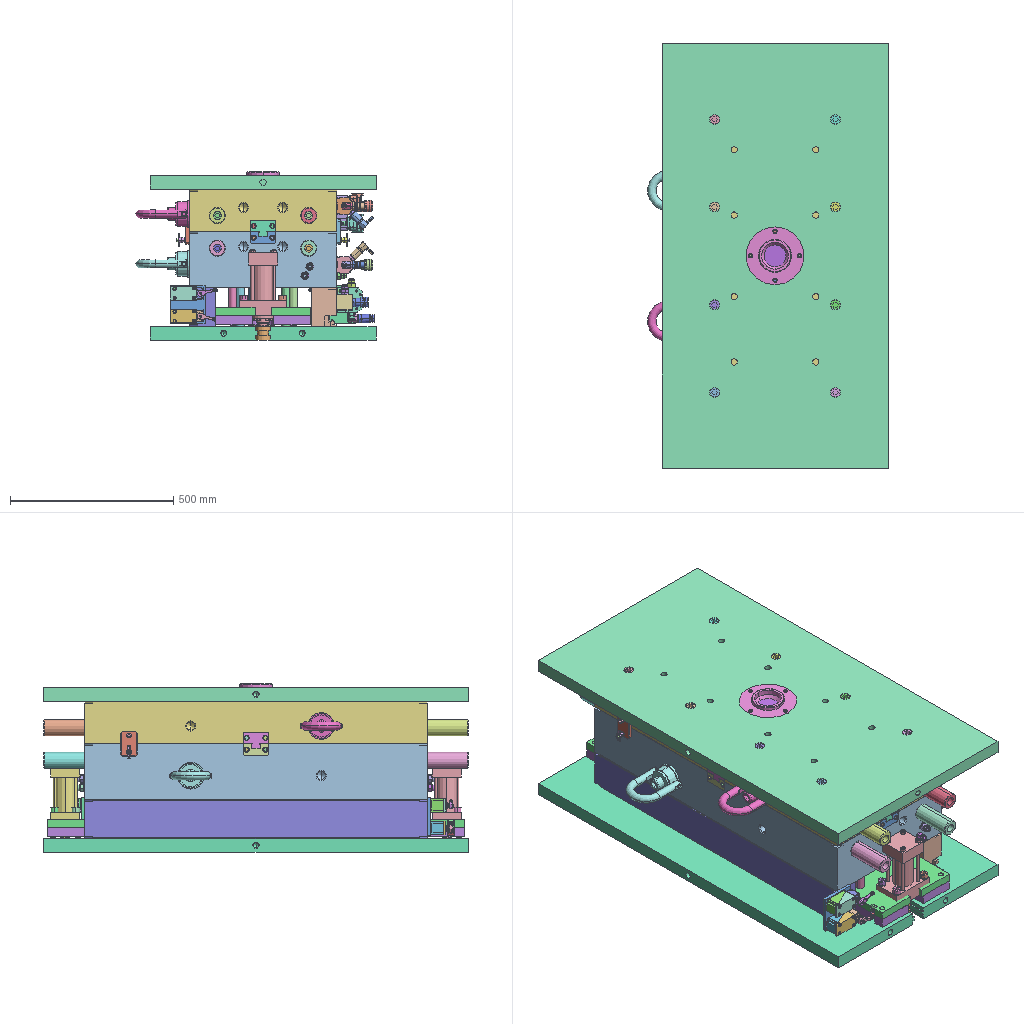Assembly | STEP file | 442 different items | 442 placed | box 735 x 1300 x 515 mm
Parts list (item | name | quantity | parent item | size | volume), first 288 of 442 items:
1 | 1 | x1 | in 4-20 | 615.081 x 1049 x 462.275 mm | 3467998 mm3
2 | 4-20.sldasm-Part-1 (subassembly) | x1 | in 4-20 | 46.6 x 158.128 x 57 mm | 97175 mm3
3 | 4-20.sldasm-Part-10 (subassembly) | x1 | in 4-20 | 14 x 7 x 7 mm | 262.874 mm3
4 | 4-20.sldasm-Part-100 (subassembly) | x1 | in 4-20 | 45.212 x 25.216 x 24.222 mm | 9310 mm3
5 | 4-20.sldasm-Part-101 (subassembly) | x1 | in 4-20 | 50 x 80 x 50 mm | 195848 mm3
6 | 4-20.sldasm-Part-102 (subassembly) | x1 | in 4-20 | 23.812 x 23.812 x 85.725 mm | 19411 mm3
7 | 4-20.sldasm-Part-103 (subassembly) | x1 | in 4-20 | 23.813 x 23.812 x 85.725 mm | 19411 mm3
8 | 4-20.sldasm-Part-104 (subassembly) | x1 | in 4-20 | 110 x 9.525 x 9.525 mm | 7838 mm3
9 | 4-20.sldasm-Part-105 (subassembly) | x1 | in 4-20 | 9.525 x 1050 x 9.525 mm | 74819 mm3
10 | 4-20.sldasm-Part-106 (subassembly) | x1 | in 4-20 | 23 x 10 x 10 mm | 863.941 mm3
11 | 4-20.sldasm-Part-107 (subassembly) | x1 | in 4-20 | 23.813 x 23.812 x 85.725 mm | 19411 mm3
12 | 4-20.sldasm-Part-108 (subassembly) | x1 | in 4-20 | 95 x 9.525 x 9.525 mm | 6769 mm3
13 | 4-20.sldasm-Part-109 (subassembly) | x1 | in 4-20 | 44.22 x 44.22 x 41.275 mm | 38759 mm3
14 | 4-20.sldasm-Part-11 (subassembly) | x1 | in 4-20 | 46.6 x 118.128 x 57 mm | 74877 mm3
15 | 4-20.sldasm-Part-110 (subassembly) | x1 | in 4-20 | 25.216 x 45.212 x 24.222 mm | 9310 mm3
16 | 4-20.sldasm-Part-111 (subassembly) | x1 | in 4-20 | 45.212 x 25.216 x 24.222 mm | 9310 mm3
17 | 4-20.sldasm-Part-112 (subassembly) | x1 | in 4-20 | 95 x 9.525 x 9.525 mm | 6769 mm3
18 | 4-20.sldasm-Part-113 (subassembly) | x1 | in 4-20 | 23 x 10 x 10 mm | 863.941 mm3
19 | 4-20.sldasm-Part-114 (subassembly) | x1 | in 4-20 | 23.813 x 23.812 x 85.725 mm | 19411 mm3
20 | 4-20.sldasm-Part-115 (subassembly) | x1 | in 4-20 | 25.216 x 45.212 x 24.222 mm | 9310 mm3
21 | 4-20.sldasm-Part-116 (subassembly) | x1 | in 4-20 | 25.216 x 45.212 x 24.222 mm | 9310 mm3
22 | 4-20.sldasm-Part-117 (subassembly) | x1 | in 4-20 | 23.813 x 23.812 x 85.725 mm | 19411 mm3
23 | 4-20.sldasm-Part-118 (subassembly) | x1 | in 4-20 | 50 x 29.094 x 26 mm | 17659 mm3
24 | 4-20.sldasm-Part-119 (subassembly) | x1 | in 4-20 | 24.222 x 25.216 x 45.212 mm | 9310 mm3
25 | 4-20.sldasm-Part-12 (subassembly) | x1 | in 4-20 | 14 x 7 x 7 mm | 262.874 mm3
26 | 4-20.sldasm-Part-120 (subassembly) | x1 | in 4-20 | 23.813 x 23.812 x 85.725 mm | 19411 mm3
27 | 4-20.sldasm-Part-121 (subassembly) | x1 | in 4-20 | 45.212 x 25.216 x 24.222 mm | 9310 mm3
28 | 4-20.sldasm-Part-122 (subassembly) | x1 | in 4-20 | 22.225 x 25.663 x 45.212 mm | 9310 mm3
29 | 4-20.sldasm-Part-123 (subassembly) | x1 | in 4-20 | 24.222 x 25.216 x 45.212 mm | 9310 mm3
30 | 4-20.sldasm-Part-124 (subassembly) | x1 | in 4-20 | 23.813 x 23.812 x 85.725 mm | 19411 mm3
31 | 4-20.sldasm-Part-125 (subassembly) | x1 | in 4-20 | 142.875 x 88.9 x 276.19 mm | 1282545 mm3
32 | 4-20.sldasm-Part-126 (subassembly) | x1 | in 4-20 | 44.22 x 44.22 x 41.275 mm | 38759 mm3
33 | 4-20.sldasm-Part-127 (subassembly) | x1 | in 4-20 | 22.225 x 25.663 x 45.212 mm | 9310 mm3
34 | 4-20.sldasm-Part-128 (subassembly) | x1 | in 4-20 | 45 x 22 x 45 mm | 14976 mm3
35 | 4-20.sldasm-Part-129 (subassembly) | x1 | in 4-20 | 79 x 192 x 94.5 mm | 576073 mm3
36 | 4-20.sldasm-Part-13 (subassembly) | x1 | in 4-20 | 14 x 7 x 7 mm | 262.874 mm3
37 | 4-20.sldasm-Part-130 (subassembly) | x1 | in 4-20 | 23 x 10 x 10 mm | 863.941 mm3
38 | 4-20.sldasm-Part-131 (subassembly) | x1 | in 4-20 | 25.216 x 45.212 x 24.222 mm | 9310 mm3
39 | 4-20.sldasm-Part-132 (subassembly) | x1 | in 4-20 | 23 x 10 x 10 mm | 863.941 mm3
40 | 4-20.sldasm-Part-133 (subassembly) | x1 | in 4-20 | 45 x 45 x 22 mm | 14976 mm3
41 | 4-20.sldasm-Part-134 (subassembly) | x1 | in 4-20 | 45.212 x 25.216 x 24.222 mm | 9310 mm3
42 | 4-20.sldasm-Part-135 (subassembly) | x1 | in 4-20 | 142.875 x 88.9 x 276.19 mm | 1282545 mm3
43 | 4-20.sldasm-Part-136 (subassembly) | x1 | in 4-20 | 59 x 10 x 10 mm | 1882 mm3
44 | 4-20.sldasm-Part-137 (subassembly) | x1 | in 4-20 | 23.812 x 23.812 x 85.725 mm | 19411 mm3
45 | 4-20.sldasm-Part-138 (subassembly) | x1 | in 4-20 | 9.525 x 1050 x 9.525 mm | 74819 mm3
46 | 4-20.sldasm-Part-139 (subassembly) | x1 | in 4-20 | 50 x 32 x 32 mm | 24309 mm3
47 | 4-20.sldasm-Part-14 (subassembly) | x1 | in 4-20 | 20 x 100 x 43 mm | 85571 mm3
48 | 4-20.sldasm-Part-140 (subassembly) | x1 | in 4-20 | 110 x 9.525 x 9.525 mm | 7838 mm3
49 | 4-20.sldasm-Part-141 (subassembly) | x1 | in 4-20 | 8.306 x 5.45 x 5.45 mm | 72.235 mm3
50 | 4-20.sldasm-Part-142 (subassembly) | x1 | in 4-20 | 3.175 x 9.6 x 3.175 mm | 75.624 mm3
51 | 4-20.sldasm-Part-143 (subassembly) | x1 | in 4-20 | 12.1 x 3.3 x 12.1 mm | 339.506 mm3
52 | 4-20.sldasm-Part-144 (subassembly) | x1 | in 4-20 | 8.306 x 5.45 x 5.45 mm | 72.196 mm3
53 | 4-20.sldasm-Part-145 (subassembly) | x1 | in 4-20 | 11.112 x 56.8 x 11.112 mm | 2501 mm3
54 | 4-20.sldasm-Part-146 (subassembly) | x1 | in 4-20 | 3.175 x 9.6 x 3.175 mm | 75.624 mm3
55 | 4-20.sldasm-Part-147 (subassembly) | x1 | in 4-20 | 9.525 x 54.15 x 9.525 mm | 1881 mm3
56 | 4-20.sldasm-Part-148 (subassembly) | x1 | in 4-20 | 7.82 x 42.968 x 7.82 mm | 439.236 mm3
57 | 4-20.sldasm-Part-149 (subassembly) | x1 | in 4-20 | 22.225 x 45.05 x 34.95 mm | 29644 mm3
58 | 4-20.sldasm-Part-15 (subassembly) | x1 | in 4-20 | 71.345 x 25 x 55.031 mm | 25800 mm3
59 | 4-20.sldasm-Part-150 (subassembly) | x1 | in 4-20 | 8.306 x 5.45 x 5.45 mm | 72.235 mm3
60 | 4-20.sldasm-Part-151 (subassembly) | x1 | in 4-20 | 20 x 15.87 x 15.87 mm | 3956 mm3
61 | 4-20.sldasm-Part-152 (subassembly) | x1 | in 4-20 | 11.112 x 56.8 x 11.112 mm | 2501 mm3
62 | 4-20.sldasm-Part-153 (subassembly) | x1 | in 4-20 | 8.306 x 5.45 x 5.45 mm | 72.196 mm3
63 | 4-20.sldasm-Part-154 (subassembly) | x1 | in 4-20 | 6.35 x 17.375 x 6.35 mm | 540.618 mm3
64 | 4-20.sldasm-Part-155 (subassembly) | x1 | in 4-20 | 6.35 x 17.375 x 6.35 mm | 540.618 mm3
65 | 4-20.sldasm-Part-156 (subassembly) | x1 | in 4-20 | 8.306 x 5.45 x 5.45 mm | 72.196 mm3
66 | 4-20.sldasm-Part-157 (subassembly) | x1 | in 4-20 | 11.112 x 56.8 x 11.112 mm | 2501 mm3
67 | 4-20.sldasm-Part-158 (subassembly) | x1 | in 4-20 | 11.113 x 56.8 x 11.112 mm | 2501 mm3
68 | 4-20.sldasm-Part-159 (subassembly) | x1 | in 4-20 | 14 x 7 x 7 mm | 258.3 mm3
69 | 4-20.sldasm-Part-16 (subassembly) | x1 | in 4-20 | 57.15 x 9.525 x 9.525 mm | 2014 mm3
70 | 4-20.sldasm-Part-160 (subassembly) | x1 | in 4-20 | 8.306 x 5.45 x 5.45 mm | 72.235 mm3
71 | 4-20.sldasm-Part-161 (subassembly) | x1 | in 4-20 | 10 x 16 x 19.5 mm | 2443 mm3
72 | 4-20.sldasm-Part-162 (subassembly) | x1 | in 4-20 | 8.306 x 5.45 x 5.45 mm | 72.235 mm3
73 | 4-20.sldasm-Part-163 (subassembly) | x1 | in 4-20 | 11.113 x 56.8 x 11.112 mm | 2501 mm3
74 | 4-20.sldasm-Part-164 (subassembly) | x1 | in 4-20 | 22.225 x 45.05 x 34.95 mm | 29644 mm3
75 | 4-20.sldasm-Part-165 (subassembly) | x1 | in 4-20 | 12.1 x 3.3 x 12.1 mm | 339.506 mm3
76 | 4-20.sldasm-Part-166 (subassembly) | x1 | in 4-20 | 8.306 x 5.45 x 5.45 mm | 72.196 mm3
77 | 4-20.sldasm-Part-167 (subassembly) | x1 | in 4-20 | 60.3 x 10 x 24.703 mm | 5847 mm3
78 | 4-20.sldasm-Part-168 (subassembly) | x1 | in 4-20 | 11.113 x 56.8 x 11.112 mm | 2501 mm3
79 | 4-20.sldasm-Part-169 (subassembly) | x1 | in 4-20 | 20 x 15.87 x 15.87 mm | 3956 mm3
80 | 4-20.sldasm-Part-17 (subassembly) | x1 | in 4-20 | 71.345 x 25 x 55.031 mm | 25800 mm3
81 | 4-20.sldasm-Part-170 (subassembly) | x1 | in 4-20 | 76.9 x 40.4 x 41.3 mm | 81109 mm3
82 | 4-20.sldasm-Part-171 (subassembly) | x1 | in 4-20 | 20 x 15.87 x 15.87 mm | 3956 mm3
83 | 4-20.sldasm-Part-172 (subassembly) | x1 | in 4-20 | 9.525 x 54.15 x 9.525 mm | 1881 mm3
84 | 4-20.sldasm-Part-173 (subassembly) | x1 | in 4-20 | 9.525 x 54.15 x 9.525 mm | 1881 mm3
85 | 4-20.sldasm-Part-174 (subassembly) | x1 | in 4-20 | 60.3 x 10 x 24.703 mm | 5847 mm3
86 | 4-20.sldasm-Part-175 (subassembly) | x1 | in 4-20 | 12.1 x 3.3 x 12.1 mm | 339.506 mm3
87 | 4-20.sldasm-Part-176 (subassembly) | x1 | in 4-20 | 11.113 x 56.8 x 11.112 mm | 2501 mm3
88 | 4-20.sldasm-Part-177 (subassembly) | x1 | in 4-20 | 8.306 x 5.45 x 5.45 mm | 72.196 mm3
89 | 4-20.sldasm-Part-178 (subassembly) | x1 | in 4-20 | 60.3 x 10 x 24.703 mm | 5847 mm3
90 | 4-20.sldasm-Part-179 (subassembly) | x1 | in 4-20 | 76.9 x 40.4 x 41.3 mm | 81109 mm3
91 | 4-20.sldasm-Part-18 (subassembly) | x1 | in 4-20 | 71.345 x 25 x 55.031 mm | 25800 mm3
92 | 4-20.sldasm-Part-180 (subassembly) | x1 | in 4-20 | 7.82 x 42.968 x 7.82 mm | 439.236 mm3
93 | 4-20.sldasm-Part-181 (subassembly) | x1 | in 4-20 | 106.7 x 10 x 117.65 mm | 125533 mm3
94 | 4-20.sldasm-Part-182 (subassembly) | x1 | in 4-20 | 8.306 x 5.45 x 5.45 mm | 72.196 mm3
95 | 4-20.sldasm-Part-183 (subassembly) | x1 | in 4-20 | 9.525 x 54.15 x 9.525 mm | 1881 mm3
96 | 4-20.sldasm-Part-184 (subassembly) | x1 | in 4-20 | 9.525 x 54.15 x 9.525 mm | 1881 mm3
97 | 4-20.sldasm-Part-185 (subassembly) | x1 | in 4-20 | 8.306 x 5.45 x 5.45 mm | 72.235 mm3
98 | 4-20.sldasm-Part-186 (subassembly) | x1 | in 4-20 | 7.82 x 12.968 x 7.82 mm | 191.707 mm3
99 | 4-20.sldasm-Part-187 (subassembly) | x1 | in 4-20 | 76.9 x 40.4 x 41.3 mm | 81109 mm3
100 | 4-20.sldasm-Part-188 (subassembly) | x1 | in 4-20 | 12.7 x 4 x 12.7 mm | 450.576 mm3
101 | 4-20.sldasm-Part-189 (subassembly) | x1 | in 4-20 | 8.306 x 5.45 x 5.45 mm | 72.196 mm3
102 | 4-20.sldasm-Part-19 (subassembly) | x1 | in 4-20 | 50.8 x 111.125 x 50.8 mm | 204378 mm3
103 | 4-20.sldasm-Part-190 (subassembly) | x1 | in 4-20 | 20 x 15.87 x 15.87 mm | 3956 mm3
104 | 4-20.sldasm-Part-191 (subassembly) | x1 | in 4-20 | 20 x 15.87 x 15.87 mm | 3956 mm3
105 | 4-20.sldasm-Part-192 (subassembly) | x1 | in 4-20 | 20 x 15.87 x 15.87 mm | 3956 mm3
106 | 4-20.sldasm-Part-193 (subassembly) | x1 | in 4-20 | 8.306 x 5.45 x 5.45 mm | 72.235 mm3
107 | 4-20.sldasm-Part-194 (subassembly) | x1 | in 4-20 | 14 x 7 x 7 mm | 258.3 mm3
108 | 4-20.sldasm-Part-195 (subassembly) | x1 | in 4-20 | 8.306 x 5.45 x 5.45 mm | 72.196 mm3
109 | 4-20.sldasm-Part-196 (subassembly) | x1 | in 4-20 | 10 x 16 x 19.5 mm | 2443 mm3
110 | 4-20.sldasm-Part-197 (subassembly) | x1 | in 4-20 | 12.7 x 4 x 12.7 mm | 450.576 mm3
111 | 4-20.sldasm-Part-198 (subassembly) | x1 | in 4-20 | 14 x 7 x 7 mm | 258.3 mm3
112 | 4-20.sldasm-Part-199 (subassembly) | x1 | in 4-20 | 12.7 x 4 x 12.7 mm | 450.576 mm3
113 | 4-20.sldasm-Part-2 (subassembly) | x1 | in 4-20 | 47 x 10 x 10 mm | 1564 mm3
114 | 4-20.sldasm-Part-20 (subassembly) | x1 | in 4-20 | 34.118 x 22.56 x 34.901 mm | 4861 mm3
115 | 4-20.sldasm-Part-200 (subassembly) | x1 | in 4-20 | 6.35 x 17.375 x 6.35 mm | 540.618 mm3
116 | 4-20.sldasm-Part-201 (subassembly) | x1 | in 4-20 | 12.1 x 3.3 x 12.1 mm | 339.506 mm3
117 | 4-20.sldasm-Part-202 (subassembly) | x1 | in 4-20 | 3.175 x 9.6 x 3.175 mm | 75.624 mm3
118 | 4-20.sldasm-Part-203 (subassembly) | x1 | in 4-20 | 11.112 x 56.8 x 11.112 mm | 2501 mm3
119 | 4-20.sldasm-Part-204 (subassembly) | x1 | in 4-20 | 60.3 x 10 x 24.703 mm | 5847 mm3
120 | 4-20.sldasm-Part-205 (subassembly) | x1 | in 4-20 | 106.7 x 10 x 117.65 mm | 125533 mm3
121 | 4-20.sldasm-Part-206 (subassembly) | x1 | in 4-20 | 9.525 x 54.15 x 9.525 mm | 1881 mm3
122 | 4-20.sldasm-Part-207 (subassembly) | x1 | in 4-20 | 22.225 x 45.05 x 34.95 mm | 29644 mm3
123 | 4-20.sldasm-Part-208 (subassembly) | x1 | in 4-20 | 8.306 x 5.45 x 5.45 mm | 72.196 mm3
124 | 4-20.sldasm-Part-209 (subassembly) | x1 | in 4-20 | 7.82 x 42.968 x 7.82 mm | 439.236 mm3
125 | 4-20.sldasm-Part-21 (subassembly) | x1 | in 4-20 | 71.345 x 25 x 55.031 mm | 25800 mm3
126 | 4-20.sldasm-Part-210 (subassembly) | x1 | in 4-20 | 22.225 x 45.05 x 34.95 mm | 29644 mm3
127 | 4-20.sldasm-Part-211 (subassembly) | x1 | in 4-20 | 81.175 x 42.9 x 41.3 mm | 66698 mm3
128 | 4-20.sldasm-Part-212 (subassembly) | x1 | in 4-20 | 8.306 x 5.45 x 5.45 mm | 72.235 mm3
129 | 4-20.sldasm-Part-213 (subassembly) | x1 | in 4-20 | 10 x 16 x 19.5 mm | 2443 mm3
130 | 4-20.sldasm-Part-214 (subassembly) | x1 | in 4-20 | 10 x 16 x 19.5 mm | 2443 mm3
131 | 4-20.sldasm-Part-215 (subassembly) | x1 | in 4-20 | 8.306 x 5.45 x 5.45 mm | 72.235 mm3
132 | 4-20.sldasm-Part-216 (subassembly) | x1 | in 4-20 | 7.82 x 12.968 x 7.82 mm | 191.707 mm3
133 | 4-20.sldasm-Part-217 (subassembly) | x1 | in 4-20 | 9.525 x 54.15 x 9.525 mm | 1881 mm3
134 | 4-20.sldasm-Part-218 (subassembly) | x1 | in 4-20 | 81.175 x 42.9 x 41.3 mm | 66698 mm3
135 | 4-20.sldasm-Part-219 (subassembly) | x1 | in 4-20 | 7.82 x 42.968 x 7.82 mm | 439.236 mm3
136 | 4-20.sldasm-Part-22 (subassembly) | x1 | in 4-20 | 50.8 x 111.125 x 50.8 mm | 204378 mm3
137 | 4-20.sldasm-Part-220 (subassembly) | x1 | in 4-20 | 9.525 x 54.15 x 9.525 mm | 1881 mm3
138 | 4-20.sldasm-Part-221 (subassembly) | x1 | in 4-20 | 12.7 x 4 x 12.7 mm | 450.576 mm3
139 | 4-20.sldasm-Part-222 (subassembly) | x1 | in 4-20 | 81.175 x 42.9 x 41.3 mm | 66698 mm3
140 | 4-20.sldasm-Part-223 (subassembly) | x1 | in 4-20 | 76.9 x 40.4 x 41.3 mm | 81109 mm3
141 | 4-20.sldasm-Part-224 (subassembly) | x1 | in 4-20 | 14 x 7 x 7 mm | 258.3 mm3
142 | 4-20.sldasm-Part-225 (subassembly) | x1 | in 4-20 | 6.35 x 17.375 x 6.35 mm | 540.618 mm3
143 | 4-20.sldasm-Part-226 (subassembly) | x1 | in 4-20 | 81.175 x 42.9 x 41.3 mm | 66698 mm3
144 | 4-20.sldasm-Part-227 (subassembly) | x1 | in 4-20 | 3.175 x 9.6 x 3.175 mm | 75.624 mm3
145 | 4-20.sldasm-Part-228 (subassembly) | x1 | in 4-20 | 8.306 x 5.45 x 5.45 mm | 72.196 mm3
146 | 4-20.sldasm-Part-229 (subassembly) | x1 | in 4-20 | 12.7 x 12.7 x 240.5 mm | 12432 mm3
147 | 4-20.sldasm-Part-23 (subassembly) | x1 | in 4-20 | 34.118 x 22.56 x 34.901 mm | 4861 mm3
148 | 4-20.sldasm-Part-230 (subassembly) | x1 | in 4-20 | 23.812 x 23.812 x 53.025 mm | 12939 mm3
149 | 4-20.sldasm-Part-231 (subassembly) | x1 | in 4-20 | 23.812 x 23.812 x 53.025 mm | 12939 mm3
150 | 4-20.sldasm-Part-232 (subassembly) | x1 | in 4-20 | 23.812 x 23.812 x 53.025 mm | 12939 mm3
151 | 4-20.sldasm-Part-233 (subassembly) | x1 | in 4-20 | 23.812 x 23.812 x 53.025 mm | 12939 mm3
152 | 4-20.sldasm-Part-234 (subassembly) | x1 | in 4-20 | 23.812 x 23.812 x 53.025 mm | 12939 mm3
153 | 4-20.sldasm-Part-235 (subassembly) | x1 | in 4-20 | 23.812 x 23.812 x 53.025 mm | 12939 mm3
154 | 4-20.sldasm-Part-236 (subassembly) | x1 | in 4-20 | 23.812 x 23.812 x 53.025 mm | 12939 mm3
155 | 4-20.sldasm-Part-237 (subassembly) | x1 | in 4-20 | 23.812 x 23.813 x 53.025 mm | 12939 mm3
156 | 4-20.sldasm-Part-238 (subassembly) | x1 | in 4-20 | 23.812 x 23.812 x 53.025 mm | 12939 mm3
157 | 4-20.sldasm-Part-239 (subassembly) | x1 | in 4-20 | 23.812 x 23.813 x 53.025 mm | 12939 mm3
158 | 4-20.sldasm-Part-24 (subassembly) | x1 | in 4-20 | 50.8 x 111.125 x 50.8 mm | 204378 mm3
159 | 4-20.sldasm-Part-240 (subassembly) | x1 | in 4-20 | 23.812 x 23.812 x 53.025 mm | 12939 mm3
160 | 4-20.sldasm-Part-241 (subassembly) | x1 | in 4-20 | 23.812 x 23.812 x 53.025 mm | 12939 mm3
161 | 4-20.sldasm-Part-242 (subassembly) | x1 | in 4-20 | 31.75 x 31.75 x 256 mm | 131075 mm3
162 | 4-20.sldasm-Part-243 (subassembly) | x1 | in 4-20 | 31.75 x 31.75 x 256 mm | 131075 mm3
163 | 4-20.sldasm-Part-244 (subassembly) | x1 | in 4-20 | 31.75 x 31.75 x 256 mm | 131075 mm3
164 | 4-20.sldasm-Part-245 (subassembly) | x1 | in 4-20 | 31.75 x 31.75 x 256 mm | 131075 mm3
165 | 4-20.sldasm-Part-246 (subassembly) | x1 | in 4-20 | 290 x 1280 x 30 mm | 9865062 mm3
166 | 4-20.sldasm-Part-247 (subassembly) | x1 | in 4-20 | 290 x 1280 x 25 mm | 7957004 mm3
167 | 4-20.sldasm-Part-248 (subassembly) | x1 | in 4-20 | 8.96 x 8.96 x 12 mm | 213.091 mm3
168 | 4-20.sldasm-Part-249 (subassembly) | x1 | in 4-20 | 8.96 x 8.96 x 12 mm | 213.091 mm3
169 | 4-20.sldasm-Part-25 (subassembly) | x1 | in 4-20 | 45 x 45 x 22 mm | 14976 mm3
170 | 4-20.sldasm-Part-250 (subassembly) | x1 | in 4-20 | 16 x 16 x 5 mm | 821.609 mm3
171 | 4-20.sldasm-Part-251 (subassembly) | x1 | in 4-20 | 16 x 16 x 5 mm | 821.609 mm3
172 | 4-20.sldasm-Part-252 (subassembly) | x1 | in 4-20 | 8.96 x 8.96 x 12 mm | 213.091 mm3
173 | 4-20.sldasm-Part-253 (subassembly) | x1 | in 4-20 | 8.96 x 8.96 x 12 mm | 213.091 mm3
174 | 4-20.sldasm-Part-254 (subassembly) | x1 | in 4-20 | 8.96 x 8.96 x 12 mm | 213.091 mm3
175 | 4-20.sldasm-Part-255 (subassembly) | x1 | in 4-20 | 16 x 16 x 5 mm | 821.609 mm3
176 | 4-20.sldasm-Part-256 (subassembly) | x1 | in 4-20 | 8.96 x 8.96 x 12 mm | 213.091 mm3
177 | 4-20.sldasm-Part-257 (subassembly) | x1 | in 4-20 | 8.96 x 8.96 x 12 mm | 213.091 mm3
178 | 4-20.sldasm-Part-258 (subassembly) | x1 | in 4-20 | 16 x 16 x 5 mm | 821.609 mm3
179 | 4-20.sldasm-Part-259 (subassembly) | x1 | in 4-20 | 8.96 x 8.96 x 12 mm | 213.091 mm3
180 | 4-20.sldasm-Part-26 (subassembly) | x1 | in 4-20 | 34.118 x 22.56 x 34.901 mm | 4861 mm3
181 | 4-20.sldasm-Part-260 (subassembly) | x1 | in 4-20 | 16 x 16 x 5 mm | 821.609 mm3
182 | 4-20.sldasm-Part-261 (subassembly) | x1 | in 4-20 | 8.96 x 8.96 x 12 mm | 213.091 mm3
183 | 4-20.sldasm-Part-262 (subassembly) | x1 | in 4-20 | 8.96 x 8.96 x 12 mm | 213.091 mm3
184 | 4-20.sldasm-Part-263 (subassembly) | x1 | in 4-20 | 8.96 x 8.96 x 12 mm | 213.091 mm3
185 | 4-20.sldasm-Part-264 (subassembly) | x1 | in 4-20 | 16 x 16 x 5 mm | 821.609 mm3
186 | 4-20.sldasm-Part-265 (subassembly) | x1 | in 4-20 | 16 x 16 x 5 mm | 821.609 mm3
187 | 4-20.sldasm-Part-266 (subassembly) | x1 | in 4-20 | 16 x 16 x 5 mm | 821.609 mm3
188 | 4-20.sldasm-Part-267 (subassembly) | x1 | in 4-20 | 8.96 x 8.96 x 12 mm | 213.091 mm3
189 | 4-20.sldasm-Part-268 (subassembly) | x1 | in 4-20 | 16 x 16 x 5 mm | 821.609 mm3
190 | 4-20.sldasm-Part-269 (subassembly) | x1 | in 4-20 | 8.96 x 8.96 x 12 mm | 213.091 mm3
191 | 4-20.sldasm-Part-27 (subassembly) | x1 | in 4-20 | 34.118 x 22.56 x 34.901 mm | 4861 mm3
192 | 4-20.sldasm-Part-270 (subassembly) | x1 | in 4-20 | 16 x 16 x 5 mm | 821.609 mm3
193 | 4-20.sldasm-Part-271 (subassembly) | x1 | in 4-20 | 8.96 x 8.96 x 12 mm | 213.091 mm3
194 | 4-20.sldasm-Part-272 (subassembly) | x1 | in 4-20 | 8.96 x 8.96 x 12 mm | 213.091 mm3
195 | 4-20.sldasm-Part-273 (subassembly) | x1 | in 4-20 | 8.96 x 8.96 x 12 mm | 213.091 mm3
196 | 4-20.sldasm-Part-274 (subassembly) | x1 | in 4-20 | 16 x 16 x 5 mm | 821.609 mm3
197 | 4-20.sldasm-Part-275 (subassembly) | x1 | in 4-20 | 16 x 16 x 5 mm | 821.609 mm3
198 | 4-20.sldasm-Part-276 (subassembly) | x1 | in 4-20 | 8.96 x 8.96 x 12 mm | 213.091 mm3
199 | 4-20.sldasm-Part-277 (subassembly) | x1 | in 4-20 | 8.96 x 8.96 x 12 mm | 213.091 mm3
200 | 4-20.sldasm-Part-278 (subassembly) | x1 | in 4-20 | 16 x 16 x 5 mm | 821.609 mm3
201 | 4-20.sldasm-Part-279 (subassembly) | x1 | in 4-20 | 16 x 16 x 5 mm | 821.609 mm3
202 | 4-20.sldasm-Part-28 (subassembly) | x1 | in 4-20 | 57.15 x 9.525 x 9.525 mm | 2014 mm3
203 | 4-20.sldasm-Part-280 (subassembly) | x1 | in 4-20 | 16 x 16 x 5 mm | 821.609 mm3
204 | 4-20.sldasm-Part-281 (subassembly) | x1 | in 4-20 | 16 x 16 x 5 mm | 821.609 mm3
205 | 4-20.sldasm-Part-282 (subassembly) | x1 | in 4-20 | 16 x 16 x 5 mm | 821.609 mm3
206 | 4-20.sldasm-Part-283 (subassembly) | x1 | in 4-20 | 16 x 16 x 5 mm | 821.609 mm3
207 | 4-20.sldasm-Part-284 (subassembly) | x1 | in 4-20 | 8.96 x 8.96 x 12 mm | 213.091 mm3
208 | 4-20.sldasm-Part-285 (subassembly) | x1 | in 4-20 | 16 x 16 x 5 mm | 821.609 mm3
209 | 4-20.sldasm-Part-286 (subassembly) | x1 | in 4-20 | 16 x 16 x 5 mm | 821.609 mm3
210 | 4-20.sldasm-Part-287 (subassembly) | x1 | in 4-20 | 16 x 16 x 5 mm | 821.609 mm3
211 | 4-20.sldasm-Part-288 (subassembly) | x1 | in 4-20 | 8.96 x 8.96 x 12 mm | 213.091 mm3
212 | 4-20.sldasm-Part-289 (subassembly) | x1 | in 4-20 | 8.96 x 8.96 x 12 mm | 213.091 mm3
213 | 4-20.sldasm-Part-29 (subassembly) | x1 | in 4-20 | 71.345 x 25 x 55.031 mm | 25800 mm3
214 | 4-20.sldasm-Part-290 (subassembly) | x1 | in 4-20 | 8.96 x 8.96 x 12 mm | 213.091 mm3
215 | 4-20.sldasm-Part-291 (subassembly) | x1 | in 4-20 | 16 x 16 x 5 mm | 821.609 mm3
216 | 4-20.sldasm-Part-292 (subassembly) | x1 | in 4-20 | 16 x 16 x 5 mm | 821.609 mm3
217 | 4-20.sldasm-Part-293 (subassembly) | x1 | in 4-20 | 8.96 x 8.96 x 12 mm | 213.091 mm3
218 | 4-20.sldasm-Part-294 (subassembly) | x1 | in 4-20 | 8.96 x 8.96 x 12 mm | 213.091 mm3
219 | 4-20.sldasm-Part-295 (subassembly) | x1 | in 4-20 | 8.96 x 8.96 x 12 mm | 213.091 mm3
220 | 4-20.sldasm-Part-296 (subassembly) | x1 | in 4-20 | 16 x 16 x 5 mm | 821.609 mm3
221 | 4-20.sldasm-Part-297 (subassembly) | x1 | in 4-20 | 16 x 16 x 5 mm | 821.609 mm3
222 | 4-20.sldasm-Part-298 (subassembly) | x1 | in 4-20 | 16 x 16 x 5 mm | 821.609 mm3
223 | 4-20.sldasm-Part-299 (subassembly) | x1 | in 4-20 | 16 x 16 x 5 mm | 821.609 mm3
224 | 4-20.sldasm-Part-3 (subassembly) | x1 | in 4-20 | 14 x 7 x 7 mm | 262.874 mm3
225 | 4-20.sldasm-Part-30 (subassembly) | x1 | in 4-20 | 63.246 x 35.458 x 35.458 mm | 27969 mm3
226 | 4-20.sldasm-Part-300 (subassembly) | x1 | in 4-20 | 8.96 x 8.96 x 12 mm | 213.091 mm3
227 | 4-20.sldasm-Part-301 (subassembly) | x1 | in 4-20 | 16 x 16 x 5 mm | 821.609 mm3
228 | 4-20.sldasm-Part-302 (subassembly) | x1 | in 4-20 | 8.96 x 8.96 x 12 mm | 213.091 mm3
229 | 4-20.sldasm-Part-303 (subassembly) | x1 | in 4-20 | 8.96 x 8.96 x 12 mm | 213.091 mm3
230 | 4-20.sldasm-Part-304 (subassembly) | x1 | in 4-20 | 8.96 x 8.96 x 12 mm | 213.091 mm3
231 | 4-20.sldasm-Part-305 (subassembly) | x1 | in 4-20 | 16 x 16 x 5 mm | 821.609 mm3
232 | 4-20.sldasm-Part-306 (subassembly) | x1 | in 4-20 | 16 x 16 x 5 mm | 821.609 mm3
233 | 4-20.sldasm-Part-307 (subassembly) | x1 | in 4-20 | 8.96 x 8.96 x 12 mm | 213.091 mm3
234 | 4-20.sldasm-Part-308 (subassembly) | x1 | in 4-20 | 28.575 x 28.575 x 196.85 mm | 60119 mm3
235 | 4-20.sldasm-Part-309 (subassembly) | x1 | in 4-20 | 23.812 x 23.813 x 73.025 mm | 16897 mm3
236 | 4-20.sldasm-Part-31 (subassembly) | x1 | in 4-20 | 57.15 x 9.525 x 9.525 mm | 2014 mm3
237 | 4-20.sldasm-Part-310 (subassembly) | x1 | in 4-20 | 28.575 x 28.575 x 196.85 mm | 60119 mm3
238 | 4-20.sldasm-Part-311 (subassembly) | x1 | in 4-20 | 28.575 x 28.575 x 196.85 mm | 60119 mm3
239 | 4-20.sldasm-Part-312 (subassembly) | x1 | in 4-20 | 23.812 x 23.812 x 73.025 mm | 16897 mm3
240 | 4-20.sldasm-Part-313 (subassembly) | x1 | in 4-20 | 28.575 x 28.575 x 196.85 mm | 60119 mm3
241 | 4-20.sldasm-Part-314 (subassembly) | x1 | in 4-20 | 23.812 x 23.812 x 73.025 mm | 16897 mm3
242 | 4-20.sldasm-Part-315 (subassembly) | x1 | in 4-20 | 28.575 x 28.575 x 196.85 mm | 60119 mm3
243 | 4-20.sldasm-Part-316 (subassembly) | x1 | in 4-20 | 23.812 x 23.812 x 73.025 mm | 16897 mm3
244 | 4-20.sldasm-Part-317 (subassembly) | x1 | in 4-20 | 28.575 x 28.575 x 196.85 mm | 60119 mm3
245 | 4-20.sldasm-Part-318 (subassembly) | x1 | in 4-20 | 28.575 x 28.575 x 196.85 mm | 60119 mm3
246 | 4-20.sldasm-Part-319 (subassembly) | x1 | in 4-20 | 23.812 x 23.812 x 73.025 mm | 16897 mm3
247 | 4-20.sldasm-Part-32 (subassembly) | x1 | in 4-20 | 63.246 x 35.458 x 35.458 mm | 27969 mm3
248 | 4-20.sldasm-Part-320 (subassembly) | x1 | in 4-20 | 23.812 x 23.813 x 73.025 mm | 16897 mm3
249 | 4-20.sldasm-Part-321 (subassembly) | x1 | in 4-20 | 28.575 x 28.575 x 196.85 mm | 60119 mm3
250 | 4-20.sldasm-Part-322 (subassembly) | x1 | in 4-20 | 60 x 60 x 120 mm | 338555 mm3
251 | 4-20.sldasm-Part-323 (subassembly) | x1 | in 4-20 | 80 x 80 x 120 mm | 602197 mm3
252 | 4-20.sldasm-Part-324 (subassembly) | x1 | in 4-20 | 60 x 60 x 120 mm | 338555 mm3
253 | 4-20.sldasm-Part-325 (subassembly) | x1 | in 4-20 | 80 x 80 x 120 mm | 602197 mm3
254 | 4-20.sldasm-Part-326 (subassembly) | x1 | in 4-20 | 60 x 60 x 120 mm | 338555 mm3
255 | 4-20.sldasm-Part-327 (subassembly) | x1 | in 4-20 | 60 x 60 x 120 mm | 338555 mm3
256 | 4-20.sldasm-Part-328 (subassembly) | x1 | in 4-20 | 692.15 x 1300 x 41.275 mm | 36129684 mm3
257 | 4-20.sldasm-Part-329 (subassembly) | x1 | in 4-20 | 78 x 1050 x 120 mm | 8694380 mm3
258 | 4-20.sldasm-Part-33 (subassembly) | x1 | in 4-20 | 71.345 x 25 x 55.031 mm | 25800 mm3
259 | 4-20.sldasm-Part-330 (subassembly) | x1 | in 4-20 | 78 x 1050 x 120 mm | 9659306 mm3
260 | 4-20.sldasm-Part-331 (subassembly) | x1 | in 4-20 | 16.088 x 16.088 x 12 mm | 2376 mm3
261 | 4-20.sldasm-Part-332 (subassembly) | x1 | in 4-20 | 12.862 x 12.862 x 22 mm | 2859 mm3
262 | 4-20.sldasm-Part-333 (subassembly) | x1 | in 4-20 | 16.088 x 12 x 16.088 mm | 2376 mm3
263 | 4-20.sldasm-Part-334 (subassembly) | x1 | in 4-20 | 16.088 x 12 x 16.088 mm | 2376 mm3
264 | 4-20.sldasm-Part-335 (subassembly) | x1 | in 4-20 | 11.11 x 380 x 11.11 mm | 36838 mm3
265 | 4-20.sldasm-Part-336 (subassembly) | x1 | in 4-20 | 11.11 x 380 x 11.11 mm | 36838 mm3
266 | 4-20.sldasm-Part-337 (subassembly) | x1 | in 4-20 | 12.862 x 12.862 x 22 mm | 2859 mm3
267 | 4-20.sldasm-Part-338 (subassembly) | x1 | in 4-20 | 12.862 x 12.862 x 22 mm | 2859 mm3
268 | 4-20.sldasm-Part-339 (subassembly) | x1 | in 4-20 | 16.088 x 12 x 16.088 mm | 2376 mm3
269 | 4-20.sldasm-Part-34 (subassembly) | x1 | in 4-20 | 34.118 x 22.56 x 34.901 mm | 4861 mm3
270 | 4-20.sldasm-Part-340 (subassembly) | x1 | in 4-20 | 11.11 x 11.11 x 50 mm | 4847 mm3
271 | 4-20.sldasm-Part-341 (subassembly) | x1 | in 4-20 | 6.35 x 292.067 x 6.35 mm | 9250 mm3
272 | 4-20.sldasm-Part-342 (subassembly) | x1 | in 4-20 | 12 x 16.088 x 16.088 mm | 2376 mm3
273 | 4-20.sldasm-Part-343 (subassembly) | x1 | in 4-20 | 11.11 x 11.11 x 50 mm | 4847 mm3
274 | 4-20.sldasm-Part-344 (subassembly) | x1 | in 4-20 | 12.862 x 12.862 x 22 mm | 2859 mm3
275 | 4-20.sldasm-Part-345 (subassembly) | x1 | in 4-20 | 175 x 11.11 x 11.11 mm | 16965 mm3
276 | 4-20.sldasm-Part-346 (subassembly) | x1 | in 4-20 | 6.35 x 292.067 x 6.35 mm | 9250 mm3
277 | 4-20.sldasm-Part-347 (subassembly) | x1 | in 4-20 | 75 x 11.11 x 11.11 mm | 7271 mm3
278 | 4-20.sldasm-Part-348 (subassembly) | x1 | in 4-20 | 11.11 x 380 x 11.11 mm | 36838 mm3
279 | 4-20.sldasm-Part-349 (subassembly) | x1 | in 4-20 | 175 x 11.11 x 11.11 mm | 16965 mm3
280 | 4-20.sldasm-Part-35 (subassembly) | x1 | in 4-20 | 71.345 x 25 x 55.031 mm | 25800 mm3
281 | 4-20.sldasm-Part-350 (subassembly) | x1 | in 4-20 | 175 x 11.11 x 11.11 mm | 16965 mm3
282 | 4-20.sldasm-Part-351 (subassembly) | x1 | in 4-20 | 75 x 11.11 x 11.11 mm | 7271 mm3
283 | 4-20.sldasm-Part-352 (subassembly) | x1 | in 4-20 | 16.088 x 12 x 16.088 mm | 2376 mm3
284 | 4-20.sldasm-Part-353 (subassembly) | x1 | in 4-20 | 11.11 x 380 x 11.11 mm | 36838 mm3
285 | 4-20.sldasm-Part-354 (subassembly) | x1 | in 4-20 | 175 x 11.11 x 11.11 mm | 16965 mm3
286 | 4-20.sldasm-Part-355 (subassembly) | x1 | in 4-20 | 12 x 16.088 x 16.088 mm | 2376 mm3
287 | 4-20.sldasm-Part-356 (subassembly) | x1 | in 4-20 | 16.088 x 16.088 x 12 mm | 2376 mm3
288 | 4-20.sldasm-Part-357 (subassembly) | x1 | in 4-20 | 19.05 x 19.05 x 82.55 mm | 11798 mm3